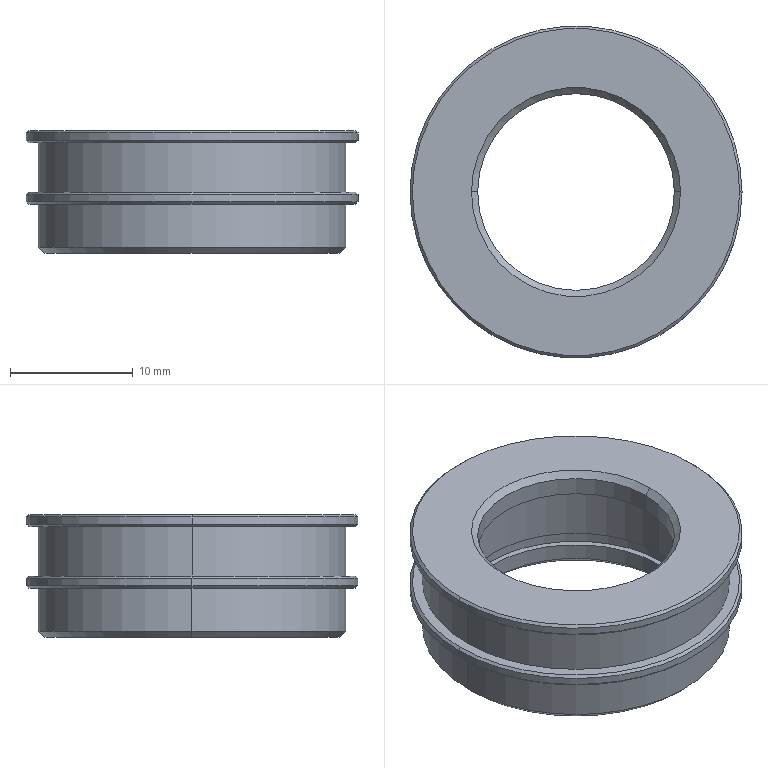Part | SolidWorks | features ICE 5, Chamfer 2, Extrusion 1 | 1 solid | 38 faces | box 27 x 27 x 10 mm | volume 2336 mm3 | cylinder 16 | cone 14 | plane 8 | commonest cylinder face diameters 19 x4 25 x4 27 x4 16 x2 20 x2
STEP:
#1=CARTESIAN_POINT('',(-13.3,0.,4.));
#2=VERTEX_POINT('',#1);
#3=CARTESIAN_POINT('',(13.3,0.,4.));
#4=VERTEX_POINT('',#3);
#5=CARTESIAN_POINT('',(0.,0.,4.));
#6=DIRECTION('',(0.,0.,-1.));
#7=DIRECTION('',(1.,0.,0.));
#8=AXIS2_PLACEMENT_3D('',#5,#6,#7);
#9=CIRCLE('',#8,13.3);
#10=EDGE_CURVE('',#2,#4,#9,.T.);
#11=ORIENTED_EDGE('',*,*,#10,.F.);
#12=CARTESIAN_POINT('',(-13.5,0.,4.2));
#13=VERTEX_POINT('',#12);
#14=CARTESIAN_POINT('',(-13.5,0.,4.2));
#15=DIRECTION('',(-0.7071,0.,0.7071));
#16=VECTOR('',#15,1000.);
#17=LINE('',#14,#16);
#18=EDGE_CURVE('',#2,#13,#17,.T.);
#19=ORIENTED_EDGE('',*,*,#18,.T.);
#20=CARTESIAN_POINT('',(13.5,0.,4.2));
#21=VERTEX_POINT('',#20);
#22=CARTESIAN_POINT('',(0.,0.,4.2));
#23=DIRECTION('',(0.,0.,1.));
#24=DIRECTION('',(1.,0.,0.));
#25=AXIS2_PLACEMENT_3D('',#22,#23,#24);
#26=CIRCLE('',#25,13.5);
#27=EDGE_CURVE('',#21,#13,#26,.T.);
#28=ORIENTED_EDGE('',*,*,#27,.F.);
#29=CARTESIAN_POINT('',(13.5,0.,4.2));
#30=DIRECTION('',(0.7071,0.,0.7071));
#31=VECTOR('',#30,1000.);
#32=LINE('',#29,#31);
#33=EDGE_CURVE('',#4,#21,#32,.T.);
#34=ORIENTED_EDGE('',*,*,#33,.F.);
#35=EDGE_LOOP('',(#11,#19,#28,#34));
#36=FACE_OUTER_BOUND('',#35,.T.);
#37=CARTESIAN_POINT('',(0.,0.,4.2));
#38=DIRECTION('',(0.,0.,1.));
#39=DIRECTION('',(1.,0.,0.));
#40=AXIS2_PLACEMENT_3D('',#37,#38,#39);
#41=CONICAL_SURFACE('',#40,13.5,0.7854);
#42=ADVANCED_FACE('',(#36),#41,.T.);
#43=CARTESIAN_POINT('',(13.3,0.,5.));
#44=VERTEX_POINT('',#43);
#45=CARTESIAN_POINT('',(-13.3,0.,5.));
#46=VERTEX_POINT('',#45);
#47=CARTESIAN_POINT('',(0.,0.,5.));
#48=DIRECTION('',(0.,0.,1.));
#49=DIRECTION('',(1.,0.,0.));
#50=AXIS2_PLACEMENT_3D('',#47,#48,#49);
#51=CIRCLE('',#50,13.3);
#52=EDGE_CURVE('',#44,#46,#51,.T.);
#53=ORIENTED_EDGE('',*,*,#52,.F.);
#54=CARTESIAN_POINT('',(13.5,0.,4.8));
#55=VERTEX_POINT('',#54);
#56=CARTESIAN_POINT('',(13.3,0.,5.));
#57=DIRECTION('',(0.7071,0.,-0.7071));
#58=VECTOR('',#57,1000.);
#59=LINE('',#56,#58);
#60=EDGE_CURVE('',#44,#55,#59,.T.);
#61=ORIENTED_EDGE('',*,*,#60,.T.);
#62=CARTESIAN_POINT('',(-13.5,0.,4.8));
#63=VERTEX_POINT('',#62);
#64=CARTESIAN_POINT('',(0.,0.,4.8));
#65=DIRECTION('',(0.,0.,-1.));
#66=DIRECTION('',(1.,0.,0.));
#67=AXIS2_PLACEMENT_3D('',#64,#65,#66);
#68=CIRCLE('',#67,13.5);
#69=EDGE_CURVE('',#63,#55,#68,.T.);
#70=ORIENTED_EDGE('',*,*,#69,.F.);
#71=CARTESIAN_POINT('',(-13.3,0.,5.));
#72=DIRECTION('',(-0.7071,0.,-0.7071));
#73=VECTOR('',#72,1000.);
#74=LINE('',#71,#73);
#75=EDGE_CURVE('',#46,#63,#74,.T.);
#76=ORIENTED_EDGE('',*,*,#75,.F.);
#77=EDGE_LOOP('',(#53,#61,#70,#76));
#78=FACE_OUTER_BOUND('',#77,.T.);
#79=CARTESIAN_POINT('',(0.,0.,5.));
#80=DIRECTION('',(0.,0.,-1.));
#81=DIRECTION('',(-1.,0.,0.));
#82=AXIS2_PLACEMENT_3D('',#79,#80,#81);
#83=CONICAL_SURFACE('',#82,13.3,0.7854);
#84=ADVANCED_FACE('',(#78),#83,.T.);
#85=CARTESIAN_POINT('',(-13.3,0.,-1.));
#86=VERTEX_POINT('',#85);
#87=CARTESIAN_POINT('',(13.3,0.,-1.));
#88=VERTEX_POINT('',#87);
#89=CARTESIAN_POINT('',(0.,0.,-1.));
#90=DIRECTION('',(0.,0.,-1.));
#91=DIRECTION('',(-1.,0.,0.));
#92=AXIS2_PLACEMENT_3D('',#89,#90,#91);
#93=CIRCLE('',#92,13.3);
#94=EDGE_CURVE('',#86,#88,#93,.T.);
#95=ORIENTED_EDGE('',*,*,#94,.F.);
#96=CARTESIAN_POINT('',(-13.5,0.,-0.8));
#97=VERTEX_POINT('',#96);
#98=CARTESIAN_POINT('',(-13.3,0.,-1.));
#99=DIRECTION('',(-0.7071,0.,0.7071));
#100=VECTOR('',#99,1000.);
#101=LINE('',#98,#100);
#102=EDGE_CURVE('',#86,#97,#101,.T.);
#103=ORIENTED_EDGE('',*,*,#102,.T.);
#104=CARTESIAN_POINT('',(13.5,0.,-0.8));
#105=VERTEX_POINT('',#104);
#106=CARTESIAN_POINT('',(0.,0.,-0.8));
#107=DIRECTION('',(0.,0.,1.));
#108=DIRECTION('',(-1.,0.,0.));
#109=AXIS2_PLACEMENT_3D('',#106,#107,#108);
#110=CIRCLE('',#109,13.5);
#111=EDGE_CURVE('',#105,#97,#110,.T.);
#112=ORIENTED_EDGE('',*,*,#111,.F.);
#113=CARTESIAN_POINT('',(13.3,0.,-1.));
#114=DIRECTION('',(0.7071,0.,0.7071));
#115=VECTOR('',#114,1000.);
#116=LINE('',#113,#115);
#117=EDGE_CURVE('',#88,#105,#116,.T.);
#118=ORIENTED_EDGE('',*,*,#117,.F.);
#119=EDGE_LOOP('',(#95,#103,#112,#118));
#120=FACE_OUTER_BOUND('',#119,.T.);
#121=CARTESIAN_POINT('',(0.,0.,-1.));
#122=DIRECTION('',(0.,0.,1.));
#123=DIRECTION('',(1.,0.,0.));
#124=AXIS2_PLACEMENT_3D('',#121,#122,#123);
#125=CONICAL_SURFACE('',#124,13.3,0.7854);
#126=ADVANCED_FACE('',(#120),#125,.T.);
#127=CARTESIAN_POINT('',(13.3,0.,0.));
#128=VERTEX_POINT('',#127);
#129=CARTESIAN_POINT('',(-13.3,0.,0.));
#130=VERTEX_POINT('',#129);
#131=CARTESIAN_POINT('',(0.,0.,0.));
#132=DIRECTION('',(0.,0.,1.));
#133=DIRECTION('',(-1.,0.,0.));
#134=AXIS2_PLACEMENT_3D('',#131,#132,#133);
#135=CIRCLE('',#134,13.3);
#136=EDGE_CURVE('',#128,#130,#135,.T.);
#137=ORIENTED_EDGE('',*,*,#136,.F.);
#138=CARTESIAN_POINT('',(13.5,0.,-0.2));
#139=VERTEX_POINT('',#138);
#140=CARTESIAN_POINT('',(13.5,0.,-0.2));
#141=DIRECTION('',(0.7071,0.,-0.7071));
#142=VECTOR('',#141,1000.);
#143=LINE('',#140,#142);
#144=EDGE_CURVE('',#128,#139,#143,.T.);
#145=ORIENTED_EDGE('',*,*,#144,.T.);
#146=CARTESIAN_POINT('',(-13.5,0.,-0.2));
#147=VERTEX_POINT('',#146);
#148=CARTESIAN_POINT('',(0.,0.,-0.2));
#149=DIRECTION('',(0.,0.,-1.));
#150=DIRECTION('',(-1.,0.,0.));
#151=AXIS2_PLACEMENT_3D('',#148,#149,#150);
#152=CIRCLE('',#151,13.5);
#153=EDGE_CURVE('',#147,#139,#152,.T.);
#154=ORIENTED_EDGE('',*,*,#153,.F.);
#155=CARTESIAN_POINT('',(-13.5,0.,-0.2));
#156=DIRECTION('',(-0.7071,0.,-0.7071));
#157=VECTOR('',#156,1000.);
#158=LINE('',#155,#157);
#159=EDGE_CURVE('',#130,#147,#158,.T.);
#160=ORIENTED_EDGE('',*,*,#159,.F.);
#161=EDGE_LOOP('',(#137,#145,#154,#160));
#162=FACE_OUTER_BOUND('',#161,.T.);
#163=CARTESIAN_POINT('',(0.,0.,-0.2));
#164=DIRECTION('',(0.,0.,-1.));
#165=DIRECTION('',(-1.,0.,0.));
#166=AXIS2_PLACEMENT_3D('',#163,#164,#165);
#167=CONICAL_SURFACE('',#166,13.5,0.7854);
#168=ADVANCED_FACE('',(#162),#167,.T.);
#169=CARTESIAN_POINT('',(-12.,0.,-5.));
#170=VERTEX_POINT('',#169);
#171=CARTESIAN_POINT('',(12.,0.,-5.));
#172=VERTEX_POINT('',#171);
#173=CARTESIAN_POINT('',(0.,0.,-5.));
#174=DIRECTION('',(0.,0.,-1.));
#175=DIRECTION('',(-1.,0.,0.));
#176=AXIS2_PLACEMENT_3D('',#173,#174,#175);
#177=CIRCLE('',#176,12.);
#178=EDGE_CURVE('',#170,#172,#177,.T.);
#179=ORIENTED_EDGE('',*,*,#178,.F.);
#180=CARTESIAN_POINT('',(-12.5,0.,-4.5));
#181=VERTEX_POINT('',#180);
#182=CARTESIAN_POINT('',(-12.,0.,-5.));
#183=DIRECTION('',(-0.7071,0.,0.7071));
#184=VECTOR('',#183,1000.);
#185=LINE('',#182,#184);
#186=EDGE_CURVE('',#170,#181,#185,.T.);
#187=ORIENTED_EDGE('',*,*,#186,.T.);
#188=CARTESIAN_POINT('',(12.5,0.,-4.5));
#189=VERTEX_POINT('',#188);
#190=CARTESIAN_POINT('',(0.,0.,-4.5));
#191=DIRECTION('',(0.,0.,1.));
#192=DIRECTION('',(-1.,0.,0.));
#193=AXIS2_PLACEMENT_3D('',#190,#191,#192);
#194=CIRCLE('',#193,12.5);
#195=EDGE_CURVE('',#189,#181,#194,.T.);
#196=ORIENTED_EDGE('',*,*,#195,.F.);
#197=CARTESIAN_POINT('',(12.,0.,-5.));
#198=DIRECTION('',(0.7071,0.,0.7071));
#199=VECTOR('',#198,1000.);
#200=LINE('',#197,#199);
#201=EDGE_CURVE('',#172,#189,#200,.T.);
#202=ORIENTED_EDGE('',*,*,#201,.F.);
#203=EDGE_LOOP('',(#179,#187,#196,#202));
#204=FACE_OUTER_BOUND('',#203,.T.);
#205=CARTESIAN_POINT('',(0.,0.,-5.));
#206=DIRECTION('',(0.,0.,1.));
#207=DIRECTION('',(1.,0.,0.));
#208=AXIS2_PLACEMENT_3D('',#205,#206,#207);
#209=CONICAL_SURFACE('',#208,12.,0.7854);
#210=ADVANCED_FACE('',(#204),#209,.T.);
#211=CARTESIAN_POINT('',(9.5,0.,-4.5));
#212=VERTEX_POINT('',#211);
#213=CARTESIAN_POINT('',(-9.5,0.,-4.5));
#214=VERTEX_POINT('',#213);
#215=CARTESIAN_POINT('',(0.,0.,-4.5));
#216=DIRECTION('',(0.,0.,-1.));
#217=DIRECTION('',(-1.,0.,0.));
#218=AXIS2_PLACEMENT_3D('',#215,#216,#217);
#219=CIRCLE('',#218,9.5);
#220=EDGE_CURVE('',#212,#214,#219,.T.);
#221=ORIENTED_EDGE('',*,*,#220,.F.);
#222=CARTESIAN_POINT('',(10.,0.,-5.));
#223=VERTEX_POINT('',#222);
#224=CARTESIAN_POINT('',(9.5,0.,-4.5));
#225=DIRECTION('',(0.7071,0.,-0.7071));
#226=VECTOR('',#225,1000.);
#227=LINE('',#224,#226);
#228=EDGE_CURVE('',#212,#223,#227,.T.);
#229=ORIENTED_EDGE('',*,*,#228,.T.);
#230=CARTESIAN_POINT('',(-10.,0.,-5.));
#231=VERTEX_POINT('',#230);
#232=CARTESIAN_POINT('',(0.,0.,-5.));
#233=DIRECTION('',(0.,0.,1.));
#234=DIRECTION('',(-1.,0.,0.));
#235=AXIS2_PLACEMENT_3D('',#232,#233,#234);
#236=CIRCLE('',#235,10.);
#237=EDGE_CURVE('',#231,#223,#236,.T.);
#238=ORIENTED_EDGE('',*,*,#237,.F.);
#239=CARTESIAN_POINT('',(-9.5,0.,-4.5));
#240=DIRECTION('',(-0.7071,0.,-0.7071));
#241=VECTOR('',#240,1000.);
#242=LINE('',#239,#241);
#243=EDGE_CURVE('',#214,#231,#242,.T.);
#244=ORIENTED_EDGE('',*,*,#243,.F.);
#245=EDGE_LOOP('',(#221,#229,#238,#244));
#246=FACE_OUTER_BOUND('',#245,.T.);
#247=CARTESIAN_POINT('',(0.,0.,-4.5));
#248=DIRECTION('',(0.,0.,-1.));
#249=DIRECTION('',(-1.,0.,0.));
#250=AXIS2_PLACEMENT_3D('',#247,#248,#249);
#251=CONICAL_SURFACE('',#250,9.5,0.7854);
#252=ADVANCED_FACE('',(#246),#251,.F.);
#253=CARTESIAN_POINT('',(-8.,0.,4.5));
#254=VERTEX_POINT('',#253);
#255=CARTESIAN_POINT('',(8.,0.,4.5));
#256=VERTEX_POINT('',#255);
#257=CARTESIAN_POINT('',(0.,0.,4.5));
#258=DIRECTION('',(0.,0.,1.));
#259=DIRECTION('',(1.,0.,0.));
#260=AXIS2_PLACEMENT_3D('',#257,#258,#259);
#261=CIRCLE('',#260,8.);
#262=EDGE_CURVE('',#254,#256,#261,.T.);
#263=ORIENTED_EDGE('',*,*,#262,.F.);
#264=CARTESIAN_POINT('',(-8.5,0.,5.));
#265=VERTEX_POINT('',#264);
#266=CARTESIAN_POINT('',(-8.,0.,4.5));
#267=DIRECTION('',(-0.7071,0.,0.7071));
#268=VECTOR('',#267,1000.);
#269=LINE('',#266,#268);
#270=EDGE_CURVE('',#254,#265,#269,.T.);
#271=ORIENTED_EDGE('',*,*,#270,.T.);
#272=CARTESIAN_POINT('',(8.5,0.,5.));
#273=VERTEX_POINT('',#272);
#274=CARTESIAN_POINT('',(0.,0.,5.));
#275=DIRECTION('',(0.,0.,-1.));
#276=DIRECTION('',(1.,0.,0.));
#277=AXIS2_PLACEMENT_3D('',#274,#275,#276);
#278=CIRCLE('',#277,8.5);
#279=EDGE_CURVE('',#273,#265,#278,.T.);
#280=ORIENTED_EDGE('',*,*,#279,.F.);
#281=CARTESIAN_POINT('',(8.,0.,4.5));
#282=DIRECTION('',(0.7071,0.,0.7071));
#283=VECTOR('',#282,1000.);
#284=LINE('',#281,#283);
#285=EDGE_CURVE('',#256,#273,#284,.T.);
#286=ORIENTED_EDGE('',*,*,#285,.F.);
#287=EDGE_LOOP('',(#263,#271,#280,#286));
#288=FACE_OUTER_BOUND('',#287,.T.);
#289=CARTESIAN_POINT('',(0.,0.,4.5));
#290=DIRECTION('',(0.,0.,1.));
#291=DIRECTION('',(1.,0.,0.));
#292=AXIS2_PLACEMENT_3D('',#289,#290,#291);
#293=CONICAL_SURFACE('',#292,8.,0.7854);
#294=ADVANCED_FACE('',(#288),#293,.F.);
#295=CARTESIAN_POINT('',(10.,0.,-3.15));
#296=VERTEX_POINT('',#295);
#297=CARTESIAN_POINT('',(-10.,0.,-3.15));
#298=VERTEX_POINT('',#297);
#299=CARTESIAN_POINT('',(0.,0.,-3.15));
#300=DIRECTION('',(0.,0.,-1.));
#301=DIRECTION('',(-1.,0.,0.));
#302=AXIS2_PLACEMENT_3D('',#299,#300,#301);
#303=CIRCLE('',#302,10.);
#304=EDGE_CURVE('',#296,#298,#303,.T.);
#305=ORIENTED_EDGE('',*,*,#304,.T.);
#306=CARTESIAN_POINT('',(-10.,0.,-2.));
#307=VERTEX_POINT('',#306);
#308=CARTESIAN_POINT('',(-10.,0.,-3.15));
#309=DIRECTION('',(0.,0.,1.));
#310=VECTOR('',#309,1000.);
#311=LINE('',#308,#310);
#312=EDGE_CURVE('',#298,#307,#311,.T.);
#313=ORIENTED_EDGE('',*,*,#312,.T.);
#314=CARTESIAN_POINT('',(10.,0.,-2.));
#315=VERTEX_POINT('',#314);
#316=CARTESIAN_POINT('',(0.,0.,-2.));
#317=DIRECTION('',(0.,0.,-1.));
#318=DIRECTION('',(-1.,0.,0.));
#319=AXIS2_PLACEMENT_3D('',#316,#317,#318);
#320=CIRCLE('',#319,10.);
#321=EDGE_CURVE('',#315,#307,#320,.T.);
#322=ORIENTED_EDGE('',*,*,#321,.F.);
#323=CARTESIAN_POINT('',(10.,0.,-3.15));
#324=DIRECTION('',(0.,0.,1.));
#325=VECTOR('',#324,1000.);
#326=LINE('',#323,#325);
#327=EDGE_CURVE('',#296,#315,#326,.T.);
#328=ORIENTED_EDGE('',*,*,#327,.F.);
#329=EDGE_LOOP('',(#305,#313,#322,#328));
#330=FACE_OUTER_BOUND('',#329,.T.);
#331=CARTESIAN_POINT('',(0.,0.,-3.15));
#332=DIRECTION('',(0.,0.,1.));
#333=DIRECTION('',(1.,0.,0.));
#334=AXIS2_PLACEMENT_3D('',#331,#332,#333);
#335=CYLINDRICAL_SURFACE('',#334,10.);
#336=ADVANCED_FACE('',(#330),#335,.F.);
#337=ORIENTED_EDGE('',*,*,#195,.T.);
#338=CARTESIAN_POINT('',(-12.5,0.,-1.));
#339=VERTEX_POINT('',#338);
#340=CARTESIAN_POINT('',(-12.5,0.,-5.));
#341=DIRECTION('',(0.,0.,1.));
#342=VECTOR('',#341,1000.);
#343=LINE('',#340,#342);
#344=EDGE_CURVE('',#181,#339,#343,.T.);
#345=ORIENTED_EDGE('',*,*,#344,.T.);
#346=CARTESIAN_POINT('',(12.5,0.,-1.));
#347=VERTEX_POINT('',#346);
#348=CARTESIAN_POINT('',(0.,0.,-1.));
#349=DIRECTION('',(0.,0.,-1.));
#350=DIRECTION('',(-1.,0.,0.));
#351=AXIS2_PLACEMENT_3D('',#348,#349,#350);
#352=CIRCLE('',#351,12.5);
#353=EDGE_CURVE('',#339,#347,#352,.T.);
#354=ORIENTED_EDGE('',*,*,#353,.T.);
#355=CARTESIAN_POINT('',(12.5,0.,-5.));
#356=DIRECTION('',(0.,0.,1.));
#357=VECTOR('',#356,1000.);
#358=LINE('',#355,#357);
#359=EDGE_CURVE('',#189,#347,#358,.T.);
#360=ORIENTED_EDGE('',*,*,#359,.F.);
#361=EDGE_LOOP('',(#337,#345,#354,#360));
#362=FACE_OUTER_BOUND('',#361,.T.);
#363=CARTESIAN_POINT('',(0.,0.,-5.));
#364=DIRECTION('',(0.,0.,1.));
#365=DIRECTION('',(1.,0.,0.));
#366=AXIS2_PLACEMENT_3D('',#363,#364,#365);
#367=CYLINDRICAL_SURFACE('',#366,12.5);
#368=ADVANCED_FACE('',(#362),#367,.T.);
#369=CARTESIAN_POINT('',(-9.5,0.,-3.15));
#370=VERTEX_POINT('',#369);
#371=CARTESIAN_POINT('',(9.5,0.,-3.15));
#372=VERTEX_POINT('',#371);
#373=CARTESIAN_POINT('',(0.,0.,-3.15));
#374=DIRECTION('',(0.,0.,1.));
#375=DIRECTION('',(-1.,0.,0.));
#376=AXIS2_PLACEMENT_3D('',#373,#374,#375);
#377=CIRCLE('',#376,9.5);
#378=EDGE_CURVE('',#370,#372,#377,.T.);
#379=ORIENTED_EDGE('',*,*,#378,.T.);
#380=CARTESIAN_POINT('',(9.5,0.,3.));
#381=DIRECTION('',(0.,0.,-1.));
#382=VECTOR('',#381,1000.);
#383=LINE('',#380,#382);
#384=EDGE_CURVE('',#372,#212,#383,.T.);
#385=ORIENTED_EDGE('',*,*,#384,.T.);
#386=ORIENTED_EDGE('',*,*,#220,.T.);
#387=CARTESIAN_POINT('',(-9.5,0.,3.));
#388=DIRECTION('',(0.,0.,-1.));
#389=VECTOR('',#388,1000.);
#390=LINE('',#387,#389);
#391=EDGE_CURVE('',#370,#214,#390,.T.);
#392=ORIENTED_EDGE('',*,*,#391,.F.);
#393=EDGE_LOOP('',(#379,#385,#386,#392));
#394=FACE_OUTER_BOUND('',#393,.T.);
#395=CARTESIAN_POINT('',(0.,0.,3.));
#396=DIRECTION('',(0.,0.,-1.));
#397=DIRECTION('',(-1.,0.,0.));
#398=AXIS2_PLACEMENT_3D('',#395,#396,#397);
#399=CYLINDRICAL_SURFACE('',#398,9.5);
#400=ADVANCED_FACE('',(#394),#399,.F.);
#401=ORIENTED_EDGE('',*,*,#111,.T.);
#402=CARTESIAN_POINT('',(-13.5,0.,-1.));
#403=DIRECTION('',(0.,0.,1.));
#404=VECTOR('',#403,1000.);
#405=LINE('',#402,#404);
#406=EDGE_CURVE('',#97,#147,#405,.T.);
#407=ORIENTED_EDGE('',*,*,#406,.T.);
#408=ORIENTED_EDGE('',*,*,#153,.T.);
#409=CARTESIAN_POINT('',(13.5,0.,-1.));
#410=DIRECTION('',(0.,0.,1.));
#411=VECTOR('',#410,1000.);
#412=LINE('',#409,#411);
#413=EDGE_CURVE('',#105,#139,#412,.T.);
#414=ORIENTED_EDGE('',*,*,#413,.F.);
#415=EDGE_LOOP('',(#401,#407,#408,#414));
#416=FACE_OUTER_BOUND('',#415,.T.);
#417=CARTESIAN_POINT('',(0.,0.,-1.));
#418=DIRECTION('',(0.,0.,1.));
#419=DIRECTION('',(1.,0.,0.));
#420=AXIS2_PLACEMENT_3D('',#417,#418,#419);
#421=CYLINDRICAL_SURFACE('',#420,13.5);
#422=ADVANCED_FACE('',(#416),#421,.T.);
#423=ORIENTED_EDGE('',*,*,#69,.T.);
#424=CARTESIAN_POINT('',(13.5,0.,5.));
#425=DIRECTION('',(0.,0.,-1.));
#426=VECTOR('',#425,1000.);
#427=LINE('',#424,#426);
#428=EDGE_CURVE('',#55,#21,#427,.T.);
#429=ORIENTED_EDGE('',*,*,#428,.T.);
#430=ORIENTED_EDGE('',*,*,#27,.T.);
#431=CARTESIAN_POINT('',(-13.5,0.,5.));
#432=DIRECTION('',(0.,0.,-1.));
#433=VECTOR('',#432,1000.);
#434=LINE('',#431,#433);
#435=EDGE_CURVE('',#63,#13,#434,.T.);
#436=ORIENTED_EDGE('',*,*,#435,.F.);
#437=EDGE_LOOP('',(#423,#429,#430,#436));
#438=FACE_OUTER_BOUND('',#437,.T.);
#439=CARTESIAN_POINT('',(0.,0.,5.));
#440=DIRECTION('',(0.,0.,-1.));
#441=DIRECTION('',(-1.,0.,0.));
#442=AXIS2_PLACEMENT_3D('',#439,#440,#441);
#443=CYLINDRICAL_SURFACE('',#442,13.5);
#444=ADVANCED_FACE('',(#438),#443,.T.);
#445=CARTESIAN_POINT('',(12.5,0.,4.));
#446=VERTEX_POINT('',#445);
#447=CARTESIAN_POINT('',(-12.5,0.,4.));
#448=VERTEX_POINT('',#447);
#449=CARTESIAN_POINT('',(0.,0.,4.));
#450=DIRECTION('',(0.,0.,1.));
#451=DIRECTION('',(1.,0.,0.));
#452=AXIS2_PLACEMENT_3D('',#449,#450,#451);
#453=CIRCLE('',#452,12.5);
#454=EDGE_CURVE('',#446,#448,#453,.T.);
#455=ORIENTED_EDGE('',*,*,#454,.F.);
#456=CARTESIAN_POINT('',(12.5,0.,0.));
#457=VERTEX_POINT('',#456);
#458=CARTESIAN_POINT('',(12.5,0.,4.));
#459=DIRECTION('',(0.,0.,-1.));
#460=VECTOR('',#459,1000.);
#461=LINE('',#458,#460);
#462=EDGE_CURVE('',#446,#457,#461,.T.);
#463=ORIENTED_EDGE('',*,*,#462,.T.);
#464=CARTESIAN_POINT('',(-12.5,0.,0.));
#465=VERTEX_POINT('',#464);
#466=CARTESIAN_POINT('',(0.,0.,0.));
#467=DIRECTION('',(0.,0.,-1.));
#468=DIRECTION('',(-1.,0.,0.));
#469=AXIS2_PLACEMENT_3D('',#466,#467,#468);
#470=CIRCLE('',#469,12.5);
#471=EDGE_CURVE('',#465,#457,#470,.T.);
#472=ORIENTED_EDGE('',*,*,#471,.F.);
#473=CARTESIAN_POINT('',(-12.5,0.,4.));
#474=DIRECTION('',(0.,0.,-1.));
#475=VECTOR('',#474,1000.);
#476=LINE('',#473,#475);
#477=EDGE_CURVE('',#448,#465,#476,.T.);
#478=ORIENTED_EDGE('',*,*,#477,.F.);
#479=EDGE_LOOP('',(#455,#463,#472,#478));
#480=FACE_OUTER_BOUND('',#479,.T.);
#481=CARTESIAN_POINT('',(0.,0.,4.));
#482=DIRECTION('',(0.,0.,-1.));
#483=DIRECTION('',(-1.,0.,0.));
#484=AXIS2_PLACEMENT_3D('',#481,#482,#483);
#485=CYLINDRICAL_SURFACE('',#484,12.5);
#486=ADVANCED_FACE('',(#480),#485,.T.);
#487=ORIENTED_EDGE('',*,*,#262,.T.);
#488=CARTESIAN_POINT('',(8.,0.,3.));
#489=VERTEX_POINT('',#488);
#490=CARTESIAN_POINT('',(8.,0.,4.));
#491=DIRECTION('',(0.,0.,-1.));
#492=VECTOR('',#491,1000.);
#493=LINE('',#490,#492);
#494=EDGE_CURVE('',#256,#489,#493,.T.);
#495=ORIENTED_EDGE('',*,*,#494,.T.);
#496=CARTESIAN_POINT('',(-8.,0.,3.));
#497=VERTEX_POINT('',#496);
#498=CARTESIAN_POINT('',(0.,0.,3.));
#499=DIRECTION('',(0.,0.,-1.));
#500=DIRECTION('',(-1.,0.,0.));
#501=AXIS2_PLACEMENT_3D('',#498,#499,#500);
#502=CIRCLE('',#501,8.);
#503=EDGE_CURVE('',#489,#497,#502,.T.);
#504=ORIENTED_EDGE('',*,*,#503,.T.);
#505=CARTESIAN_POINT('',(-8.,0.,4.));
#506=DIRECTION('',(0.,0.,-1.));
#507=VECTOR('',#506,1000.);
#508=LINE('',#505,#507);
#509=EDGE_CURVE('',#254,#497,#508,.T.);
#510=ORIENTED_EDGE('',*,*,#509,.F.);
#511=EDGE_LOOP('',(#487,#495,#504,#510));
#512=FACE_OUTER_BOUND('',#511,.T.);
#513=CARTESIAN_POINT('',(0.,0.,4.));
#514=DIRECTION('',(0.,0.,-1.));
#515=DIRECTION('',(-1.,0.,0.));
#516=AXIS2_PLACEMENT_3D('',#513,#514,#515);
#517=CYLINDRICAL_SURFACE('',#516,8.);
#518=ADVANCED_FACE('',(#512),#517,.F.);
#519=CARTESIAN_POINT('',(9.5,0.,3.));
#520=VERTEX_POINT('',#519);
#521=CARTESIAN_POINT('',(-9.5,0.,3.));
#522=VERTEX_POINT('',#521);
#523=CARTESIAN_POINT('',(0.,0.,3.));
#524=DIRECTION('',(0.,0.,-1.));
#525=DIRECTION('',(-1.,0.,0.));
#526=AXIS2_PLACEMENT_3D('',#523,#524,#525);
#527=CIRCLE('',#526,9.5);
#528=EDGE_CURVE('',#520,#522,#527,.T.);
#529=ORIENTED_EDGE('',*,*,#528,.F.);
#530=CARTESIAN_POINT('',(9.5,0.,-2.));
#531=VERTEX_POINT('',#530);
#532=CARTESIAN_POINT('',(9.5,0.,3.));
#533=DIRECTION('',(0.,0.,-1.));
#534=VECTOR('',#533,1000.);
#535=LINE('',#532,#534);
#536=EDGE_CURVE('',#520,#531,#535,.T.);
#537=ORIENTED_EDGE('',*,*,#536,.T.);
#538=CARTESIAN_POINT('',(-9.5,0.,-2.));
#539=VERTEX_POINT('',#538);
#540=CARTESIAN_POINT('',(0.,0.,-2.));
#541=DIRECTION('',(0.,0.,1.));
#542=DIRECTION('',(-1.,0.,0.));
#543=AXIS2_PLACEMENT_3D('',#540,#541,#542);
#544=CIRCLE('',#543,9.5);
#545=EDGE_CURVE('',#539,#531,#544,.T.);
#546=ORIENTED_EDGE('',*,*,#545,.F.);
#547=CARTESIAN_POINT('',(-9.5,0.,3.));
#548=DIRECTION('',(0.,0.,-1.));
#549=VECTOR('',#548,1000.);
#550=LINE('',#547,#549);
#551=EDGE_CURVE('',#522,#539,#550,.T.);
#552=ORIENTED_EDGE('',*,*,#551,.F.);
#553=EDGE_LOOP('',(#529,#537,#546,#552));
#554=FACE_OUTER_BOUND('',#553,.T.);
#555=CARTESIAN_POINT('',(0.,0.,3.));
#556=DIRECTION('',(0.,0.,-1.));
#557=DIRECTION('',(-1.,0.,0.));
#558=AXIS2_PLACEMENT_3D('',#555,#556,#557);
#559=CYLINDRICAL_SURFACE('',#558,9.5);
#560=ADVANCED_FACE('',(#554),#559,.F.);
#561=ORIENTED_EDGE('',*,*,#536,.F.);
#562=CARTESIAN_POINT('',(0.,0.,3.));
#563=DIRECTION('',(0.,0.,-1.));
#564=DIRECTION('',(-1.,0.,0.));
#565=AXIS2_PLACEMENT_3D('',#562,#563,#564);
#566=CIRCLE('',#565,9.5);
#567=EDGE_CURVE('',#522,#520,#566,.T.);
#568=ORIENTED_EDGE('',*,*,#567,.F.);
#569=ORIENTED_EDGE('',*,*,#551,.T.);
#570=CARTESIAN_POINT('',(0.,0.,-2.));
#571=DIRECTION('',(0.,0.,1.));
#572=DIRECTION('',(-1.,0.,0.));
#573=AXIS2_PLACEMENT_3D('',#570,#571,#572);
#574=CIRCLE('',#573,9.5);
#575=EDGE_CURVE('',#531,#539,#574,.T.);
#576=ORIENTED_EDGE('',*,*,#575,.F.);
#577=EDGE_LOOP('',(#561,#568,#569,#576));
#578=FACE_OUTER_BOUND('',#577,.T.);
#579=CARTESIAN_POINT('',(0.,0.,3.));
#580=DIRECTION('',(0.,0.,-1.));
#581=DIRECTION('',(-1.,0.,0.));
#582=AXIS2_PLACEMENT_3D('',#579,#580,#581);
#583=CYLINDRICAL_SURFACE('',#582,9.5);
#584=ADVANCED_FACE('',(#578),#583,.F.);
#585=CARTESIAN_POINT('',(0.,0.,-1.));
#586=DIRECTION('',(0.,0.,-1.));
#587=DIRECTION('',(-1.,0.,0.));
#588=AXIS2_PLACEMENT_3D('',#585,#586,#587);
#589=CIRCLE('',#588,13.3);
#590=EDGE_CURVE('',#88,#86,#589,.T.);
#591=ORIENTED_EDGE('',*,*,#590,.T.);
#592=ORIENTED_EDGE('',*,*,#94,.T.);
#593=EDGE_LOOP('',(#591,#592));
#594=FACE_OUTER_BOUND('',#593,.T.);
#595=CARTESIAN_POINT('',(0.,0.,-1.));
#596=DIRECTION('',(0.,0.,-1.));
#597=DIRECTION('',(-1.,0.,0.));
#598=AXIS2_PLACEMENT_3D('',#595,#596,#597);
#599=CIRCLE('',#598,12.5);
#600=EDGE_CURVE('',#347,#339,#599,.T.);
#601=ORIENTED_EDGE('',*,*,#600,.F.);
#602=ORIENTED_EDGE('',*,*,#353,.F.);
#603=EDGE_LOOP('',(#601,#602));
#604=FACE_BOUND('',#603,.T.);
#605=CARTESIAN_POINT('',(0.,0.,-1.));
#606=DIRECTION('',(0.,0.,-1.));
#607=DIRECTION('',(-1.,0.,0.));
#608=AXIS2_PLACEMENT_3D('',#605,#606,#607);
#609=PLANE('',#608);
#610=ADVANCED_FACE('',(#594,#604),#609,.T.);
#611=ORIENTED_EDGE('',*,*,#494,.F.);
#612=CARTESIAN_POINT('',(0.,0.,4.5));
#613=DIRECTION('',(0.,0.,1.));
#614=DIRECTION('',(1.,0.,0.));
#615=AXIS2_PLACEMENT_3D('',#612,#613,#614);
#616=CIRCLE('',#615,8.);
#617=EDGE_CURVE('',#256,#254,#616,.T.);
#618=ORIENTED_EDGE('',*,*,#617,.T.);
#619=ORIENTED_EDGE('',*,*,#509,.T.);
#620=CARTESIAN_POINT('',(0.,0.,3.));
#621=DIRECTION('',(0.,0.,-1.));
#622=DIRECTION('',(-1.,0.,0.));
#623=AXIS2_PLACEMENT_3D('',#620,#621,#622);
#624=CIRCLE('',#623,8.);
#625=EDGE_CURVE('',#497,#489,#624,.T.);
#626=ORIENTED_EDGE('',*,*,#625,.T.);
#627=EDGE_LOOP('',(#611,#618,#619,#626));
#628=FACE_OUTER_BOUND('',#627,.T.);
#629=CARTESIAN_POINT('',(0.,0.,4.));
#630=DIRECTION('',(0.,0.,-1.));
#631=DIRECTION('',(-1.,0.,0.));
#632=AXIS2_PLACEMENT_3D('',#629,#630,#631);
#633=CYLINDRICAL_SURFACE('',#632,8.);
#634=ADVANCED_FACE('',(#628),#633,.F.);
#635=ORIENTED_EDGE('',*,*,#462,.F.);
#636=CARTESIAN_POINT('',(0.,0.,4.));
#637=DIRECTION('',(0.,0.,1.));
#638=DIRECTION('',(1.,0.,0.));
#639=AXIS2_PLACEMENT_3D('',#636,#637,#638);
#640=CIRCLE('',#639,12.5);
#641=EDGE_CURVE('',#448,#446,#640,.T.);
#642=ORIENTED_EDGE('',*,*,#641,.F.);
#643=ORIENTED_EDGE('',*,*,#477,.T.);
#644=CARTESIAN_POINT('',(0.,0.,0.));
#645=DIRECTION('',(0.,0.,-1.));
#646=DIRECTION('',(-1.,0.,0.));
#647=AXIS2_PLACEMENT_3D('',#644,#645,#646);
#648=CIRCLE('',#647,12.5);
#649=EDGE_CURVE('',#457,#465,#648,.T.);
#650=ORIENTED_EDGE('',*,*,#649,.F.);
#651=EDGE_LOOP('',(#635,#642,#643,#650));
#652=FACE_OUTER_BOUND('',#651,.T.);
#653=CARTESIAN_POINT('',(0.,0.,4.));
#654=DIRECTION('',(0.,0.,-1.));
#655=DIRECTION('',(-1.,0.,0.));
#656=AXIS2_PLACEMENT_3D('',#653,#654,#655);
#657=CYLINDRICAL_SURFACE('',#656,12.5);
#658=ADVANCED_FACE('',(#652),#657,.T.);
#659=CARTESIAN_POINT('',(0.,0.,4.));
#660=DIRECTION('',(0.,0.,-1.));
#661=DIRECTION('',(1.,0.,0.));
#662=AXIS2_PLACEMENT_3D('',#659,#660,#661);
#663=CIRCLE('',#662,13.3);
#664=EDGE_CURVE('',#4,#2,#663,.T.);
#665=ORIENTED_EDGE('',*,*,#664,.T.);
#666=ORIENTED_EDGE('',*,*,#10,.T.);
#667=EDGE_LOOP('',(#665,#666));
#668=FACE_OUTER_BOUND('',#667,.T.);
#669=ORIENTED_EDGE('',*,*,#641,.T.);
#670=ORIENTED_EDGE('',*,*,#454,.T.);
#671=EDGE_LOOP('',(#669,#670));
#672=FACE_BOUND('',#671,.T.);
#673=CARTESIAN_POINT('',(0.,0.,4.));
#674=DIRECTION('',(0.,0.,1.));
#675=DIRECTION('',(1.,0.,0.));
#676=AXIS2_PLACEMENT_3D('',#673,#674,#675);
#677=PLANE('',#676);
#678=ADVANCED_FACE('',(#668,#672),#677,.F.);
#679=CARTESIAN_POINT('',(0.,0.,5.));
#680=DIRECTION('',(0.,0.,1.));
#681=DIRECTION('',(1.,0.,0.));
#682=AXIS2_PLACEMENT_3D('',#679,#680,#681);
#683=CIRCLE('',#682,13.3);
#684=EDGE_CURVE('',#46,#44,#683,.T.);
#685=ORIENTED_EDGE('',*,*,#684,.T.);
#686=ORIENTED_EDGE('',*,*,#52,.T.);
#687=EDGE_LOOP('',(#685,#686));
#688=FACE_OUTER_BOUND('',#687,.T.);
#689=ORIENTED_EDGE('',*,*,#279,.T.);
#690=CARTESIAN_POINT('',(0.,0.,5.));
#691=DIRECTION('',(0.,0.,-1.));
#692=DIRECTION('',(1.,0.,0.));
#693=AXIS2_PLACEMENT_3D('',#690,#691,#692);
#694=CIRCLE('',#693,8.5);
#695=EDGE_CURVE('',#265,#273,#694,.T.);
#696=ORIENTED_EDGE('',*,*,#695,.T.);
#697=EDGE_LOOP('',(#689,#696));
#698=FACE_BOUND('',#697,.T.);
#699=CARTESIAN_POINT('',(0.,0.,5.));
#700=DIRECTION('',(0.,0.,1.));
#701=DIRECTION('',(1.,0.,0.));
#702=AXIS2_PLACEMENT_3D('',#699,#700,#701);
#703=PLANE('',#702);
#704=ADVANCED_FACE('',(#688,#698),#703,.T.);
#705=ORIENTED_EDGE('',*,*,#428,.F.);
#706=CARTESIAN_POINT('',(0.,0.,4.8));
#707=DIRECTION('',(0.,0.,-1.));
#708=DIRECTION('',(1.,0.,0.));
#709=AXIS2_PLACEMENT_3D('',#706,#707,#708);
#710=CIRCLE('',#709,13.5);
#711=EDGE_CURVE('',#55,#63,#710,.T.);
#712=ORIENTED_EDGE('',*,*,#711,.T.);
#713=ORIENTED_EDGE('',*,*,#435,.T.);
#714=CARTESIAN_POINT('',(0.,0.,4.2));
#715=DIRECTION('',(0.,0.,1.));
#716=DIRECTION('',(1.,0.,0.));
#717=AXIS2_PLACEMENT_3D('',#714,#715,#716);
#718=CIRCLE('',#717,13.5);
#719=EDGE_CURVE('',#13,#21,#718,.T.);
#720=ORIENTED_EDGE('',*,*,#719,.T.);
#721=EDGE_LOOP('',(#705,#712,#713,#720));
#722=FACE_OUTER_BOUND('',#721,.T.);
#723=CARTESIAN_POINT('',(0.,0.,5.));
#724=DIRECTION('',(0.,0.,-1.));
#725=DIRECTION('',(-1.,0.,0.));
#726=AXIS2_PLACEMENT_3D('',#723,#724,#725);
#727=CYLINDRICAL_SURFACE('',#726,13.5);
#728=ADVANCED_FACE('',(#722),#727,.T.);
#729=CARTESIAN_POINT('',(0.,0.,0.));
#730=DIRECTION('',(0.,0.,1.));
#731=DIRECTION('',(-1.,0.,0.));
#732=AXIS2_PLACEMENT_3D('',#729,#730,#731);
#733=CIRCLE('',#732,13.3);
#734=EDGE_CURVE('',#130,#128,#733,.T.);
#735=ORIENTED_EDGE('',*,*,#734,.T.);
#736=ORIENTED_EDGE('',*,*,#136,.T.);
#737=EDGE_LOOP('',(#735,#736));
#738=FACE_OUTER_BOUND('',#737,.T.);
#739=ORIENTED_EDGE('',*,*,#471,.T.);
#740=ORIENTED_EDGE('',*,*,#649,.T.);
#741=EDGE_LOOP('',(#739,#740));
#742=FACE_BOUND('',#741,.T.);
#743=CARTESIAN_POINT('',(0.,0.,0.));
#744=DIRECTION('',(0.,0.,-1.));
#745=DIRECTION('',(-1.,0.,0.));
#746=AXIS2_PLACEMENT_3D('',#743,#744,#745);
#747=PLANE('',#746);
#748=ADVANCED_FACE('',(#738,#742),#747,.F.);
#749=ORIENTED_EDGE('',*,*,#406,.F.);
#750=CARTESIAN_POINT('',(0.,0.,-0.8));
#751=DIRECTION('',(0.,0.,1.));
#752=DIRECTION('',(-1.,0.,0.));
#753=AXIS2_PLACEMENT_3D('',#750,#751,#752);
#754=CIRCLE('',#753,13.5);
#755=EDGE_CURVE('',#97,#105,#754,.T.);
#756=ORIENTED_EDGE('',*,*,#755,.T.);
#757=ORIENTED_EDGE('',*,*,#413,.T.);
#758=CARTESIAN_POINT('',(0.,0.,-0.2));
#759=DIRECTION('',(0.,0.,-1.));
#760=DIRECTION('',(-1.,0.,0.));
#761=AXIS2_PLACEMENT_3D('',#758,#759,#760);
#762=CIRCLE('',#761,13.5);
#763=EDGE_CURVE('',#139,#147,#762,.T.);
#764=ORIENTED_EDGE('',*,*,#763,.T.);
#765=EDGE_LOOP('',(#749,#756,#757,#764));
#766=FACE_OUTER_BOUND('',#765,.T.);
#767=CARTESIAN_POINT('',(0.,0.,-1.));
#768=DIRECTION('',(0.,0.,1.));
#769=DIRECTION('',(1.,0.,0.));
#770=AXIS2_PLACEMENT_3D('',#767,#768,#769);
#771=CYLINDRICAL_SURFACE('',#770,13.5);
#772=ADVANCED_FACE('',(#766),#771,.T.);
#773=ORIENTED_EDGE('',*,*,#384,.F.);
#774=CARTESIAN_POINT('',(0.,0.,-3.15));
#775=DIRECTION('',(0.,0.,1.));
#776=DIRECTION('',(-1.,0.,0.));
#777=AXIS2_PLACEMENT_3D('',#774,#775,#776);
#778=CIRCLE('',#777,9.5);
#779=EDGE_CURVE('',#372,#370,#778,.T.);
#780=ORIENTED_EDGE('',*,*,#779,.T.);
#781=ORIENTED_EDGE('',*,*,#391,.T.);
#782=CARTESIAN_POINT('',(0.,0.,-4.5));
#783=DIRECTION('',(0.,0.,-1.));
#784=DIRECTION('',(-1.,0.,0.));
#785=AXIS2_PLACEMENT_3D('',#782,#783,#784);
#786=CIRCLE('',#785,9.5);
#787=EDGE_CURVE('',#214,#212,#786,.T.);
#788=ORIENTED_EDGE('',*,*,#787,.T.);
#789=EDGE_LOOP('',(#773,#780,#781,#788));
#790=FACE_OUTER_BOUND('',#789,.T.);
#791=CARTESIAN_POINT('',(0.,0.,3.));
#792=DIRECTION('',(0.,0.,-1.));
#793=DIRECTION('',(-1.,0.,0.));
#794=AXIS2_PLACEMENT_3D('',#791,#792,#793);
#795=CYLINDRICAL_SURFACE('',#794,9.5);
#796=ADVANCED_FACE('',(#790),#795,.F.);
#797=ORIENTED_EDGE('',*,*,#625,.F.);
#798=ORIENTED_EDGE('',*,*,#503,.F.);
#799=EDGE_LOOP('',(#797,#798));
#800=FACE_BOUND('',#799,.T.);
#801=ORIENTED_EDGE('',*,*,#567,.T.);
#802=ORIENTED_EDGE('',*,*,#528,.T.);
#803=EDGE_LOOP('',(#801,#802));
#804=FACE_OUTER_BOUND('',#803,.T.);
#805=CARTESIAN_POINT('',(0.,0.,3.));
#806=DIRECTION('',(0.,0.,-1.));
#807=DIRECTION('',(-1.,0.,0.));
#808=AXIS2_PLACEMENT_3D('',#805,#806,#807);
#809=PLANE('',#808);
#810=ADVANCED_FACE('',(#800,#804),#809,.T.);
#811=ORIENTED_EDGE('',*,*,#237,.T.);
#812=CARTESIAN_POINT('',(0.,0.,-5.));
#813=DIRECTION('',(0.,0.,1.));
#814=DIRECTION('',(-1.,0.,0.));
#815=AXIS2_PLACEMENT_3D('',#812,#813,#814);
#816=CIRCLE('',#815,10.);
#817=EDGE_CURVE('',#223,#231,#816,.T.);
#818=ORIENTED_EDGE('',*,*,#817,.T.);
#819=EDGE_LOOP('',(#811,#818));
#820=FACE_BOUND('',#819,.T.);
#821=CARTESIAN_POINT('',(0.,0.,-5.));
#822=DIRECTION('',(0.,0.,-1.));
#823=DIRECTION('',(-1.,0.,0.));
#824=AXIS2_PLACEMENT_3D('',#821,#822,#823);
#825=CIRCLE('',#824,12.);
#826=EDGE_CURVE('',#172,#170,#825,.T.);
#827=ORIENTED_EDGE('',*,*,#826,.T.);
#828=ORIENTED_EDGE('',*,*,#178,.T.);
#829=EDGE_LOOP('',(#827,#828));
#830=FACE_OUTER_BOUND('',#829,.T.);
#831=CARTESIAN_POINT('',(0.,0.,-5.));
#832=DIRECTION('',(0.,0.,-1.));
#833=DIRECTION('',(-1.,0.,0.));
#834=AXIS2_PLACEMENT_3D('',#831,#832,#833);
#835=PLANE('',#834);
#836=ADVANCED_FACE('',(#820,#830),#835,.T.);
#837=ORIENTED_EDGE('',*,*,#344,.F.);
#838=CARTESIAN_POINT('',(0.,0.,-4.5));
#839=DIRECTION('',(0.,0.,1.));
#840=DIRECTION('',(-1.,0.,0.));
#841=AXIS2_PLACEMENT_3D('',#838,#839,#840);
#842=CIRCLE('',#841,12.5);
#843=EDGE_CURVE('',#181,#189,#842,.T.);
#844=ORIENTED_EDGE('',*,*,#843,.T.);
#845=ORIENTED_EDGE('',*,*,#359,.T.);
#846=ORIENTED_EDGE('',*,*,#600,.T.);
#847=EDGE_LOOP('',(#837,#844,#845,#846));
#848=FACE_OUTER_BOUND('',#847,.T.);
#849=CARTESIAN_POINT('',(0.,0.,-5.));
#850=DIRECTION('',(0.,0.,1.));
#851=DIRECTION('',(1.,0.,0.));
#852=AXIS2_PLACEMENT_3D('',#849,#850,#851);
#853=CYLINDRICAL_SURFACE('',#852,12.5);
#854=ADVANCED_FACE('',(#848),#853,.T.);
#855=ORIENTED_EDGE('',*,*,#304,.F.);
#856=CARTESIAN_POINT('',(0.,0.,-3.15));
#857=DIRECTION('',(0.,0.,-1.));
#858=DIRECTION('',(-1.,0.,0.));
#859=AXIS2_PLACEMENT_3D('',#856,#857,#858);
#860=CIRCLE('',#859,10.);
#861=EDGE_CURVE('',#298,#296,#860,.T.);
#862=ORIENTED_EDGE('',*,*,#861,.F.);
#863=EDGE_LOOP('',(#855,#862));
#864=FACE_OUTER_BOUND('',#863,.T.);
#865=ORIENTED_EDGE('',*,*,#378,.F.);
#866=ORIENTED_EDGE('',*,*,#779,.F.);
#867=EDGE_LOOP('',(#865,#866));
#868=FACE_BOUND('',#867,.T.);
#869=CARTESIAN_POINT('',(0.,0.,-3.15));
#870=DIRECTION('',(0.,0.,-1.));
#871=DIRECTION('',(-1.,0.,0.));
#872=AXIS2_PLACEMENT_3D('',#869,#870,#871);
#873=PLANE('',#872);
#874=ADVANCED_FACE('',(#864,#868),#873,.F.);
#875=ORIENTED_EDGE('',*,*,#321,.T.);
#876=CARTESIAN_POINT('',(0.,0.,-2.));
#877=DIRECTION('',(0.,0.,-1.));
#878=DIRECTION('',(-1.,0.,0.));
#879=AXIS2_PLACEMENT_3D('',#876,#877,#878);
#880=CIRCLE('',#879,10.);
#881=EDGE_CURVE('',#307,#315,#880,.T.);
#882=ORIENTED_EDGE('',*,*,#881,.T.);
#883=EDGE_LOOP('',(#875,#882));
#884=FACE_OUTER_BOUND('',#883,.T.);
#885=ORIENTED_EDGE('',*,*,#545,.T.);
#886=ORIENTED_EDGE('',*,*,#575,.T.);
#887=EDGE_LOOP('',(#885,#886));
#888=FACE_BOUND('',#887,.T.);
#889=CARTESIAN_POINT('',(0.,0.,-2.));
#890=DIRECTION('',(0.,0.,-1.));
#891=DIRECTION('',(-1.,0.,0.));
#892=AXIS2_PLACEMENT_3D('',#889,#890,#891);
#893=PLANE('',#892);
#894=ADVANCED_FACE('',(#884,#888),#893,.T.);
#895=ORIENTED_EDGE('',*,*,#312,.F.);
#896=ORIENTED_EDGE('',*,*,#861,.T.);
#897=ORIENTED_EDGE('',*,*,#327,.T.);
#898=ORIENTED_EDGE('',*,*,#881,.F.);
#899=EDGE_LOOP('',(#895,#896,#897,#898));
#900=FACE_OUTER_BOUND('',#899,.T.);
#901=CARTESIAN_POINT('',(0.,0.,-3.15));
#902=DIRECTION('',(0.,0.,1.));
#903=DIRECTION('',(1.,0.,0.));
#904=AXIS2_PLACEMENT_3D('',#901,#902,#903);
#905=CYLINDRICAL_SURFACE('',#904,10.);
#906=ADVANCED_FACE('',(#900),#905,.F.);
#907=ORIENTED_EDGE('',*,*,#270,.F.);
#908=ORIENTED_EDGE('',*,*,#617,.F.);
#909=ORIENTED_EDGE('',*,*,#285,.T.);
#910=ORIENTED_EDGE('',*,*,#695,.F.);
#911=EDGE_LOOP('',(#907,#908,#909,#910));
#912=FACE_OUTER_BOUND('',#911,.T.);
#913=CARTESIAN_POINT('',(0.,0.,4.5));
#914=DIRECTION('',(0.,0.,1.));
#915=DIRECTION('',(1.,0.,0.));
#916=AXIS2_PLACEMENT_3D('',#913,#914,#915);
#917=CONICAL_SURFACE('',#916,8.,0.7854);
#918=ADVANCED_FACE('',(#912),#917,.F.);
#919=ORIENTED_EDGE('',*,*,#228,.F.);
#920=ORIENTED_EDGE('',*,*,#787,.F.);
#921=ORIENTED_EDGE('',*,*,#243,.T.);
#922=ORIENTED_EDGE('',*,*,#817,.F.);
#923=EDGE_LOOP('',(#919,#920,#921,#922));
#924=FACE_OUTER_BOUND('',#923,.T.);
#925=CARTESIAN_POINT('',(0.,0.,-4.5));
#926=DIRECTION('',(0.,0.,-1.));
#927=DIRECTION('',(-1.,0.,0.));
#928=AXIS2_PLACEMENT_3D('',#925,#926,#927);
#929=CONICAL_SURFACE('',#928,9.5,0.7854);
#930=ADVANCED_FACE('',(#924),#929,.F.);
#931=ORIENTED_EDGE('',*,*,#186,.F.);
#932=ORIENTED_EDGE('',*,*,#826,.F.);
#933=ORIENTED_EDGE('',*,*,#201,.T.);
#934=ORIENTED_EDGE('',*,*,#843,.F.);
#935=EDGE_LOOP('',(#931,#932,#933,#934));
#936=FACE_OUTER_BOUND('',#935,.T.);
#937=CARTESIAN_POINT('',(0.,0.,-5.));
#938=DIRECTION('',(0.,0.,1.));
#939=DIRECTION('',(1.,0.,0.));
#940=AXIS2_PLACEMENT_3D('',#937,#938,#939);
#941=CONICAL_SURFACE('',#940,12.,0.7854);
#942=ADVANCED_FACE('',(#936),#941,.T.);
#943=ORIENTED_EDGE('',*,*,#144,.F.);
#944=ORIENTED_EDGE('',*,*,#734,.F.);
#945=ORIENTED_EDGE('',*,*,#159,.T.);
#946=ORIENTED_EDGE('',*,*,#763,.F.);
#947=EDGE_LOOP('',(#943,#944,#945,#946));
#948=FACE_OUTER_BOUND('',#947,.T.);
#949=CARTESIAN_POINT('',(0.,0.,-0.2));
#950=DIRECTION('',(0.,0.,-1.));
#951=DIRECTION('',(-1.,0.,0.));
#952=AXIS2_PLACEMENT_3D('',#949,#950,#951);
#953=CONICAL_SURFACE('',#952,13.5,0.7854);
#954=ADVANCED_FACE('',(#948),#953,.T.);
#955=ORIENTED_EDGE('',*,*,#102,.F.);
#956=ORIENTED_EDGE('',*,*,#590,.F.);
#957=ORIENTED_EDGE('',*,*,#117,.T.);
#958=ORIENTED_EDGE('',*,*,#755,.F.);
#959=EDGE_LOOP('',(#955,#956,#957,#958));
#960=FACE_OUTER_BOUND('',#959,.T.);
#961=CARTESIAN_POINT('',(0.,0.,-1.));
#962=DIRECTION('',(0.,0.,1.));
#963=DIRECTION('',(1.,0.,0.));
#964=AXIS2_PLACEMENT_3D('',#961,#962,#963);
#965=CONICAL_SURFACE('',#964,13.3,0.7854);
#966=ADVANCED_FACE('',(#960),#965,.T.);
#967=ORIENTED_EDGE('',*,*,#60,.F.);
#968=ORIENTED_EDGE('',*,*,#684,.F.);
#969=ORIENTED_EDGE('',*,*,#75,.T.);
#970=ORIENTED_EDGE('',*,*,#711,.F.);
#971=EDGE_LOOP('',(#967,#968,#969,#970));
#972=FACE_OUTER_BOUND('',#971,.T.);
#973=CARTESIAN_POINT('',(0.,0.,5.));
#974=DIRECTION('',(0.,0.,-1.));
#975=DIRECTION('',(-1.,0.,0.));
#976=AXIS2_PLACEMENT_3D('',#973,#974,#975);
#977=CONICAL_SURFACE('',#976,13.3,0.7854);
#978=ADVANCED_FACE('',(#972),#977,.T.);
#979=ORIENTED_EDGE('',*,*,#18,.F.);
#980=ORIENTED_EDGE('',*,*,#664,.F.);
#981=ORIENTED_EDGE('',*,*,#33,.T.);
#982=ORIENTED_EDGE('',*,*,#719,.F.);
#983=EDGE_LOOP('',(#979,#980,#981,#982));
#984=FACE_OUTER_BOUND('',#983,.T.);
#985=CARTESIAN_POINT('',(0.,0.,4.2));
#986=DIRECTION('',(0.,0.,1.));
#987=DIRECTION('',(1.,0.,0.));
#988=AXIS2_PLACEMENT_3D('',#985,#986,#987);
#989=CONICAL_SURFACE('',#988,13.5,0.7854);
#990=ADVANCED_FACE('',(#984),#989,.T.);
#991=CLOSED_SHELL('',(#42,#84,#126,#168,#210,#252,#294,#336,#368,#400,#422,#444,#486,#518,#560,#584,#610,#634,#658,#678,#704,#728,#748,#772,#796,#810,#836,#854,#874,#894,#906,#918,#930,#942,#954,#966,#978,#990));
#992=MANIFOLD_SOLID_BREP('',#991);
#993=CARTESIAN_POINT('',(0.,0.,0.));
#994=DIRECTION('',(0.,0.,1.));
#995=DIRECTION('',(1.,0.,0.));
#996=AXIS2_PLACEMENT_3D('',#993,#994,#995);
#997=(LENGTH_UNIT()NAMED_UNIT(*)SI_UNIT(.MILLI.,.METRE.));
#998=UNCERTAINTY_MEASURE_WITH_UNIT(LENGTH_MEASURE(0.00001),#997,'','');
#999=(NAMED_UNIT(*)PLANE_ANGLE_UNIT()SI_UNIT($,.RADIAN.));
#1000=(NAMED_UNIT(*)SI_UNIT($,.STERADIAN.)SOLID_ANGLE_UNIT());
#1001=(GEOMETRIC_REPRESENTATION_CONTEXT(3)GLOBAL_UNCERTAINTY_ASSIGNED_CONTEXT((#998))GLOBAL_UNIT_ASSIGNED_CONTEXT((#997,#999,#1000))REPRESENTATION_CONTEXT('',''));
#1002=ADVANCED_BREP_SHAPE_REPRESENTATION('',(#992,#996),#1001);